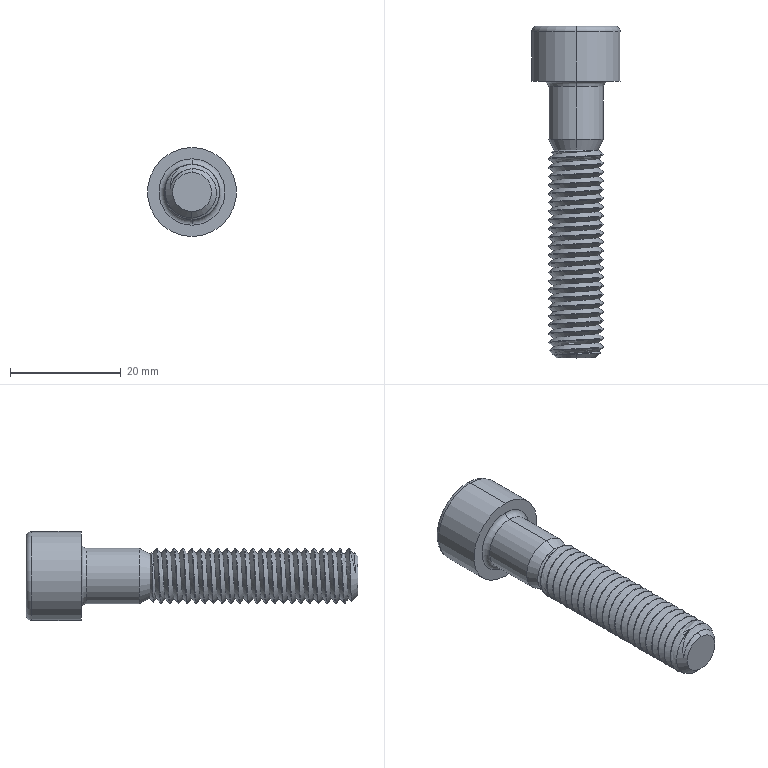Part | STEP file | Parafuso M10 - 50mm | 1 solid | 77 faces | box 16.1 x 60 x 16.1 mm | volume 4992 mm3 | cylinder 50 | plane 10 | cone 9 | torus 6 | spline 2 | commonest cylinder face diameters 10 x48 16.1 x2